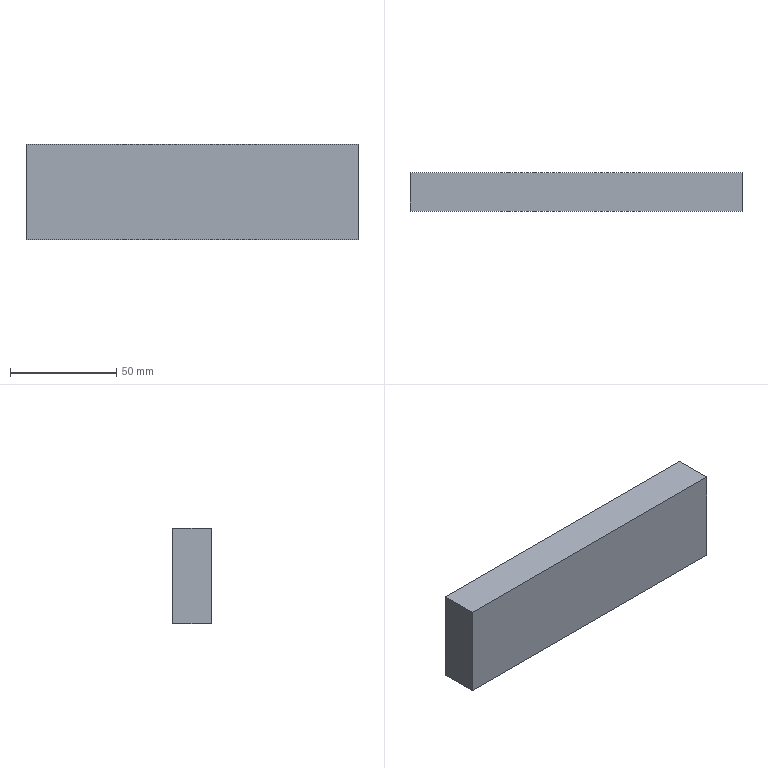CAM job | NX | 3-axis milling | part box 156 x 18 x 45 mm | stock box 156 x 18 x 45 mm
Tools:
number,name,description,diameter,corner_radius,flute_length,length,flutes
1,D16C,,16.0,0.0,50.0,75.0,2
2,D14J,,14.0,0.0,50.0,75.0,2
3,D4C,,4.0,0.0,50.0,75.0,2
4,D4J,,4.0,0.0,50.0,75.0,2
5,D4DJ,,4.0,0.0,50.0,75.0,2
6,D8C,,8.0,0.0,50.0,75.0,2
7,D6J,,6.0,0.0,50.0,75.0,2
Operations:
program,operation,operation_type,tool,method,geometry_group,spindle_rpm,surface_speed,feed_per_tooth,feed_cut,feed_plunge,cut_length_mm,path_length_mm,cut_time_min,machine_time_min
G54,PLANAR_MILL,PlanarMilling,D16C,METHOD,WORKPIECE,2300.0,115.0,0.1739,800.0,100.0,186.0,220.0,0.2325,0.2359
G54,ADAPTIVE_MILLING,CavityMilling,D16C,METHOD,WORKPIECE,3500.0,175.0,0.2143,1500.0,100.0,5345.4,5461.4,2.623,2.634
G54,PLANAR_MILL_1,PlanarMilling,D14J,METHOD,WORKPIECE,3000.0,131.0,0.1,600.0,100.0,758.357,876.357,1.264,1.276
G54,PLANAR_MILL_1_COPY_1,PlanarMilling,D14J,METHOD,WORKPIECE,3000.0,131.0,0.1,600.0,100.0,55.566,311.893,0.0926,0.1182
G54,PLANAR_MILL_2,PlanarMilling,D4C,METHOD,WORKPIECE,3500.0,43.0,0.2143,1500.0,100.0,13415.432,13465.432,8.944,8.949
G54,PLANAR_MILL_2_COPY,PlanarMilling,D4J,METHOD,WORKPIECE,3500.0,43.0,0.0571,400.0,100.0,970.275,1074.691,2.426,2.436
G54,PLANAR_MILL_2_COPY_COPY,PlanarMilling,D4DJ,METHOD,WORKPIECE,3500.0,43.0,0.1429,1000.0,100.0,250.38,288.38,0.2504,0.2542
G54,PLANAR_MILL_1_COPY,PlanarMilling,D4DJ,METHOD,WORKPIECE,3000.0,131.0,0.1,600.0,100.0,341.566,379.566,0.5693,0.5731
G54,PLANAR_MILL_3,PlanarMilling,D4DJ,METHOD,WORKPIECE,3500.0,43.0,0.1429,1000.0,100.0,95.74,446.442,0.0957,0.1308
G55,PLANAR_PROFILING,PlanarMilling,D8C,METHOD,G55,3500.0,87.0,0.2857,2000.0,100.0,12293.036,12351.176,6.146,6.152
G55,PLANAR_PROFILING_COPY,PlanarMilling,D6J,METHOD,G55,3000.0,37.0,0.0667,400.0,100.0,199.092,257.032,0.4977,0.5035
G55,FLOOR_WALL,VolumeBased25DMillingOperation,D4C,METHOD,G55,3500.0,43.0,0.2143,1500.0,100.0,2047.437,2113.664,1.365,1.372
G55,PLANAR_MILL_4,PlanarMilling,D4C,METHOD,G55,3500.0,43.0,0.2143,1500.0,100.0,4975.709,5027.079,3.317,3.322
G55,FLOOR_WALL_COPY,VolumeBased25DMillingOperation,D4J,METHOD,G55,3000.0,37.0,0.0667,400.0,100.0,97.497,141.597,0.2437,0.2482
G55,PLANAR_MILL_4_COPY,PlanarMilling,D4J,METHOD,G55,3500.0,43.0,0.2143,1500.0,100.0,128.58,189.32,0.0857,0.0918
G55,PLANAR_MILL_5_COPY_1,PlanarMilling,D4DJ,METHOD,G55,3000.0,37.0,0.1667,1000.0,100.0,207.539,245.279,0.2075,0.2113
G55,PLANAR_MILL_5_COPY,PlanarMilling,D4DJ,METHOD,G55,3000.0,37.0,0.1667,1000.0,100.0,73.779,111.779,0.0738,0.0776
G55,PLANAR_MILL_5,PlanarMilling,D4DJ,METHOD,G55,3000.0,37.0,0.1667,1000.0,100.0,121.436,159.176,0.1214,0.1252